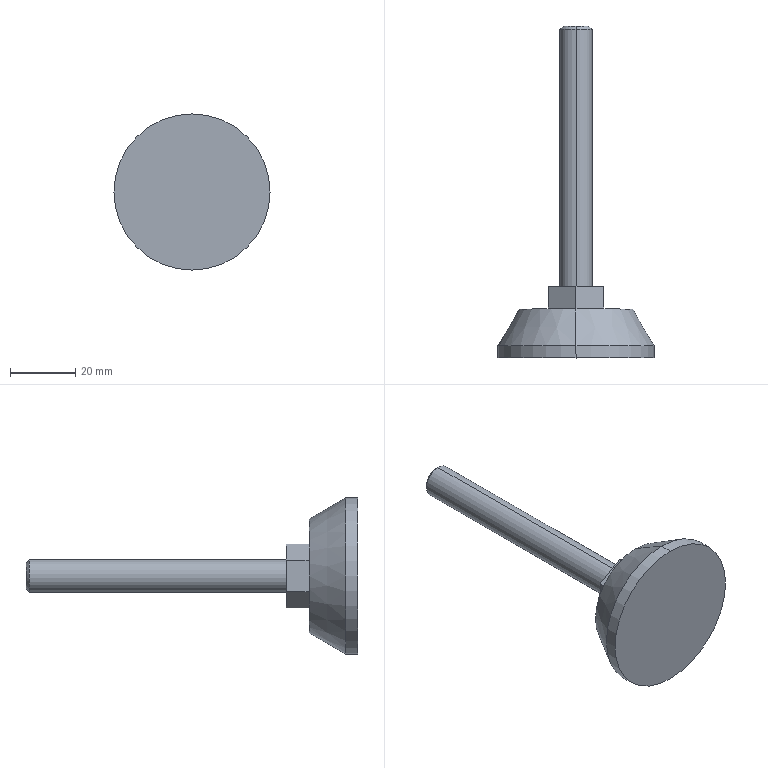Part | STEP file | AJC-D48-M10-L80 | 1 solid | 18 faces | box 48 x 102 x 48 mm | volume 30151 mm3 | plane 10 | cylinder 4 | cone 4 | commonest cylinder face diameters 10 x2 48 x2
STEP:
#1=CARTESIAN_POINT('',(0.,3.75,-24.));
#2=VERTEX_POINT('',#1);
#3=CARTESIAN_POINT('',(0.,3.75,24.));
#4=VERTEX_POINT('',#3);
#5=CARTESIAN_POINT('',(0.,3.75,0.));
#6=DIRECTION('',(0.,-1.,0.));
#7=DIRECTION('',(0.,0.,-1.));
#8=AXIS2_PLACEMENT_3D('',#5,#6,#7);
#9=CIRCLE('',#8,24.);
#10=EDGE_CURVE('',#2,#4,#9,.T.);
#11=ORIENTED_EDGE('',*,*,#10,.T.);
#12=CARTESIAN_POINT('',(0.,0.,24.));
#13=VERTEX_POINT('',#12);
#14=CARTESIAN_POINT('',(0.,107.1,24.));
#15=DIRECTION('',(0.,-1.,0.));
#16=VECTOR('',#15,1000.);
#17=LINE('',#14,#16);
#18=EDGE_CURVE('',#4,#13,#17,.T.);
#19=ORIENTED_EDGE('',*,*,#18,.T.);
#20=CARTESIAN_POINT('',(0.,0.,-24.));
#21=VERTEX_POINT('',#20);
#22=CARTESIAN_POINT('',(0.,0.,0.));
#23=DIRECTION('',(0.,-1.,0.));
#24=DIRECTION('',(0.,0.,-1.));
#25=AXIS2_PLACEMENT_3D('',#22,#23,#24);
#26=CIRCLE('',#25,24.);
#27=EDGE_CURVE('',#21,#13,#26,.T.);
#28=ORIENTED_EDGE('',*,*,#27,.F.);
#29=CARTESIAN_POINT('',(0.,107.1,-24.));
#30=DIRECTION('',(0.,-1.,0.));
#31=VECTOR('',#30,1000.);
#32=LINE('',#29,#31);
#33=EDGE_CURVE('',#2,#21,#32,.T.);
#34=ORIENTED_EDGE('',*,*,#33,.F.);
#35=EDGE_LOOP('',(#11,#19,#28,#34));
#36=FACE_OUTER_BOUND('',#35,.T.);
#37=CARTESIAN_POINT('',(0.,107.1,0.));
#38=DIRECTION('',(0.,-1.,0.));
#39=DIRECTION('',(0.,0.,-1.));
#40=AXIS2_PLACEMENT_3D('',#37,#38,#39);
#41=CYLINDRICAL_SURFACE('',#40,24.);
#42=ADVANCED_FACE('',(#36),#41,.T.);
#43=CARTESIAN_POINT('',(0.,15.,-17.505));
#44=VERTEX_POINT('',#43);
#45=CARTESIAN_POINT('',(0.,15.,17.505));
#46=VERTEX_POINT('',#45);
#47=CARTESIAN_POINT('',(0.,15.,0.));
#48=DIRECTION('',(0.,-1.,0.));
#49=DIRECTION('',(0.,0.,-1.));
#50=AXIS2_PLACEMENT_3D('',#47,#48,#49);
#51=CIRCLE('',#50,17.505);
#52=EDGE_CURVE('',#44,#46,#51,.T.);
#53=ORIENTED_EDGE('',*,*,#52,.T.);
#54=CARTESIAN_POINT('',(0.,3.75,24.));
#55=DIRECTION('',(0.,-0.866,0.5));
#56=VECTOR('',#55,1000.);
#57=LINE('',#54,#56);
#58=EDGE_CURVE('',#46,#4,#57,.T.);
#59=ORIENTED_EDGE('',*,*,#58,.T.);
#60=ORIENTED_EDGE('',*,*,#10,.F.);
#61=CARTESIAN_POINT('',(0.,3.75,-24.));
#62=DIRECTION('',(0.,-0.866,-0.5));
#63=VECTOR('',#62,1000.);
#64=LINE('',#61,#63);
#65=EDGE_CURVE('',#44,#2,#64,.T.);
#66=ORIENTED_EDGE('',*,*,#65,.F.);
#67=EDGE_LOOP('',(#53,#59,#60,#66));
#68=FACE_OUTER_BOUND('',#67,.T.);
#69=CARTESIAN_POINT('',(0.,3.75,0.));
#70=DIRECTION('',(0.,-1.,0.));
#71=DIRECTION('',(0.,0.,-1.));
#72=AXIS2_PLACEMENT_3D('',#69,#70,#71);
#73=CONICAL_SURFACE('',#72,24.,0.5236);
#74=ADVANCED_FACE('',(#68),#73,.T.);
#75=CARTESIAN_POINT('',(0.,101.,-5.));
#76=VERTEX_POINT('',#75);
#77=CARTESIAN_POINT('',(0.,101.,5.));
#78=VERTEX_POINT('',#77);
#79=CARTESIAN_POINT('',(0.,101.,0.));
#80=DIRECTION('',(0.,-1.,0.));
#81=DIRECTION('',(0.,0.,-1.));
#82=AXIS2_PLACEMENT_3D('',#79,#80,#81);
#83=CIRCLE('',#82,5.);
#84=EDGE_CURVE('',#76,#78,#83,.T.);
#85=ORIENTED_EDGE('',*,*,#84,.T.);
#86=CARTESIAN_POINT('',(0.,22.,5.));
#87=VERTEX_POINT('',#86);
#88=CARTESIAN_POINT('',(0.,107.1,5.));
#89=DIRECTION('',(0.,-1.,0.));
#90=VECTOR('',#89,1000.);
#91=LINE('',#88,#90);
#92=EDGE_CURVE('',#78,#87,#91,.T.);
#93=ORIENTED_EDGE('',*,*,#92,.T.);
#94=CARTESIAN_POINT('',(0.,22.,-5.));
#95=VERTEX_POINT('',#94);
#96=CARTESIAN_POINT('',(0.,22.,0.));
#97=DIRECTION('',(0.,1.,0.));
#98=DIRECTION('',(0.,0.,-1.));
#99=AXIS2_PLACEMENT_3D('',#96,#97,#98);
#100=CIRCLE('',#99,5.);
#101=EDGE_CURVE('',#87,#95,#100,.T.);
#102=ORIENTED_EDGE('',*,*,#101,.T.);
#103=CARTESIAN_POINT('',(0.,107.1,-5.));
#104=DIRECTION('',(0.,-1.,0.));
#105=VECTOR('',#104,1000.);
#106=LINE('',#103,#105);
#107=EDGE_CURVE('',#76,#95,#106,.T.);
#108=ORIENTED_EDGE('',*,*,#107,.F.);
#109=EDGE_LOOP('',(#85,#93,#102,#108));
#110=FACE_OUTER_BOUND('',#109,.T.);
#111=CARTESIAN_POINT('',(0.,107.1,0.));
#112=DIRECTION('',(0.,-1.,0.));
#113=DIRECTION('',(0.,0.,-1.));
#114=AXIS2_PLACEMENT_3D('',#111,#112,#113);
#115=CYLINDRICAL_SURFACE('',#114,5.);
#116=ADVANCED_FACE('',(#110),#115,.T.);
#117=CARTESIAN_POINT('',(0.,102.,-4.));
#118=VERTEX_POINT('',#117);
#119=CARTESIAN_POINT('',(0.,102.,4.));
#120=VERTEX_POINT('',#119);
#121=CARTESIAN_POINT('',(0.,102.,0.));
#122=DIRECTION('',(0.,-1.,0.));
#123=DIRECTION('',(0.,0.,-1.));
#124=AXIS2_PLACEMENT_3D('',#121,#122,#123);
#125=CIRCLE('',#124,4.);
#126=EDGE_CURVE('',#118,#120,#125,.T.);
#127=ORIENTED_EDGE('',*,*,#126,.T.);
#128=CARTESIAN_POINT('',(0.,101.,5.));
#129=DIRECTION('',(0.,-0.7071,0.7071));
#130=VECTOR('',#129,1000.);
#131=LINE('',#128,#130);
#132=EDGE_CURVE('',#120,#78,#131,.T.);
#133=ORIENTED_EDGE('',*,*,#132,.T.);
#134=ORIENTED_EDGE('',*,*,#84,.F.);
#135=CARTESIAN_POINT('',(0.,101.,-5.));
#136=DIRECTION('',(0.,-0.7071,-0.7071));
#137=VECTOR('',#136,1000.);
#138=LINE('',#135,#137);
#139=EDGE_CURVE('',#118,#76,#138,.T.);
#140=ORIENTED_EDGE('',*,*,#139,.F.);
#141=EDGE_LOOP('',(#127,#133,#134,#140));
#142=FACE_OUTER_BOUND('',#141,.T.);
#143=CARTESIAN_POINT('',(0.,101.,0.));
#144=DIRECTION('',(0.,-1.,0.));
#145=DIRECTION('',(0.,0.,-1.));
#146=AXIS2_PLACEMENT_3D('',#143,#144,#145);
#147=CONICAL_SURFACE('',#146,5.,0.7854);
#148=ADVANCED_FACE('',(#142),#147,.T.);
#149=ORIENTED_EDGE('',*,*,#27,.T.);
#150=CARTESIAN_POINT('',(0.,0.,0.));
#151=DIRECTION('',(0.,-1.,0.));
#152=DIRECTION('',(0.,0.,-1.));
#153=AXIS2_PLACEMENT_3D('',#150,#151,#152);
#154=CIRCLE('',#153,24.);
#155=EDGE_CURVE('',#13,#21,#154,.T.);
#156=ORIENTED_EDGE('',*,*,#155,.T.);
#157=EDGE_LOOP('',(#149,#156));
#158=FACE_OUTER_BOUND('',#157,.T.);
#159=CARTESIAN_POINT('',(0.,0.,0.));
#160=DIRECTION('',(0.,-1.,0.));
#161=DIRECTION('',(0.,0.,-1.));
#162=AXIS2_PLACEMENT_3D('',#159,#160,#161);
#163=PLANE('',#162);
#164=ADVANCED_FACE('',(#158),#163,.T.);
#165=ORIENTED_EDGE('',*,*,#18,.F.);
#166=CARTESIAN_POINT('',(0.,3.75,0.));
#167=DIRECTION('',(0.,-1.,0.));
#168=DIRECTION('',(0.,0.,-1.));
#169=AXIS2_PLACEMENT_3D('',#166,#167,#168);
#170=CIRCLE('',#169,24.);
#171=EDGE_CURVE('',#4,#2,#170,.T.);
#172=ORIENTED_EDGE('',*,*,#171,.T.);
#173=ORIENTED_EDGE('',*,*,#33,.T.);
#174=ORIENTED_EDGE('',*,*,#155,.F.);
#175=EDGE_LOOP('',(#165,#172,#173,#174));
#176=FACE_OUTER_BOUND('',#175,.T.);
#177=CARTESIAN_POINT('',(0.,107.1,0.));
#178=DIRECTION('',(0.,-1.,0.));
#179=DIRECTION('',(0.,0.,-1.));
#180=AXIS2_PLACEMENT_3D('',#177,#178,#179);
#181=CYLINDRICAL_SURFACE('',#180,24.);
#182=ADVANCED_FACE('',(#176),#181,.T.);
#183=ORIENTED_EDGE('',*,*,#58,.F.);
#184=CARTESIAN_POINT('',(0.,15.,0.));
#185=DIRECTION('',(0.,-1.,0.));
#186=DIRECTION('',(0.,0.,-1.));
#187=AXIS2_PLACEMENT_3D('',#184,#185,#186);
#188=CIRCLE('',#187,17.505);
#189=EDGE_CURVE('',#46,#44,#188,.T.);
#190=ORIENTED_EDGE('',*,*,#189,.T.);
#191=ORIENTED_EDGE('',*,*,#65,.T.);
#192=ORIENTED_EDGE('',*,*,#171,.F.);
#193=EDGE_LOOP('',(#183,#190,#191,#192));
#194=FACE_OUTER_BOUND('',#193,.T.);
#195=CARTESIAN_POINT('',(0.,3.75,0.));
#196=DIRECTION('',(0.,-1.,0.));
#197=DIRECTION('',(0.,0.,-1.));
#198=AXIS2_PLACEMENT_3D('',#195,#196,#197);
#199=CONICAL_SURFACE('',#198,24.,0.5236);
#200=ADVANCED_FACE('',(#194),#199,.T.);
#201=CARTESIAN_POINT('',(8.5,15.,4.907));
#202=VERTEX_POINT('',#201);
#203=CARTESIAN_POINT('',(8.5,15.,-4.907));
#204=VERTEX_POINT('',#203);
#205=CARTESIAN_POINT('',(8.5,15.,0.));
#206=DIRECTION('',(0.,0.,-1.));
#207=VECTOR('',#206,1000.);
#208=LINE('',#205,#207);
#209=EDGE_CURVE('',#202,#204,#208,.T.);
#210=ORIENTED_EDGE('',*,*,#209,.F.);
#211=CARTESIAN_POINT('',(0.,15.,9.815));
#212=VERTEX_POINT('',#211);
#213=CARTESIAN_POINT('',(0.,15.,9.815));
#214=DIRECTION('',(0.866,0.,-0.5));
#215=VECTOR('',#214,1000.);
#216=LINE('',#213,#215);
#217=EDGE_CURVE('',#212,#202,#216,.T.);
#218=ORIENTED_EDGE('',*,*,#217,.F.);
#219=CARTESIAN_POINT('',(-8.5,15.,4.907));
#220=VERTEX_POINT('',#219);
#221=CARTESIAN_POINT('',(-8.5,15.,4.907));
#222=DIRECTION('',(0.866,0.,0.5));
#223=VECTOR('',#222,1000.);
#224=LINE('',#221,#223);
#225=EDGE_CURVE('',#220,#212,#224,.T.);
#226=ORIENTED_EDGE('',*,*,#225,.F.);
#227=CARTESIAN_POINT('',(-8.5,15.,-4.907));
#228=VERTEX_POINT('',#227);
#229=CARTESIAN_POINT('',(-8.5,15.,0.));
#230=DIRECTION('',(0.,0.,1.));
#231=VECTOR('',#230,1000.);
#232=LINE('',#229,#231);
#233=EDGE_CURVE('',#228,#220,#232,.T.);
#234=ORIENTED_EDGE('',*,*,#233,.F.);
#235=CARTESIAN_POINT('',(0.,15.,-9.815));
#236=VERTEX_POINT('',#235);
#237=CARTESIAN_POINT('',(0.,15.,-9.815));
#238=DIRECTION('',(-0.866,0.,0.5));
#239=VECTOR('',#238,1000.);
#240=LINE('',#237,#239);
#241=EDGE_CURVE('',#236,#228,#240,.T.);
#242=ORIENTED_EDGE('',*,*,#241,.F.);
#243=CARTESIAN_POINT('',(8.5,15.,-4.907));
#244=DIRECTION('',(-0.866,0.,-0.5));
#245=VECTOR('',#244,1000.);
#246=LINE('',#243,#245);
#247=EDGE_CURVE('',#204,#236,#246,.T.);
#248=ORIENTED_EDGE('',*,*,#247,.F.);
#249=EDGE_LOOP('',(#210,#218,#226,#234,#242,#248));
#250=FACE_BOUND('',#249,.T.);
#251=ORIENTED_EDGE('',*,*,#52,.F.);
#252=ORIENTED_EDGE('',*,*,#189,.F.);
#253=EDGE_LOOP('',(#251,#252));
#254=FACE_OUTER_BOUND('',#253,.T.);
#255=CARTESIAN_POINT('',(0.,15.,0.));
#256=DIRECTION('',(0.,-1.,0.));
#257=DIRECTION('',(0.,0.,-1.));
#258=AXIS2_PLACEMENT_3D('',#255,#256,#257);
#259=PLANE('',#258);
#260=ADVANCED_FACE('',(#250,#254),#259,.F.);
#261=CARTESIAN_POINT('',(8.5,22.,-4.907));
#262=VERTEX_POINT('',#261);
#263=CARTESIAN_POINT('',(8.5,22.,-4.907));
#264=DIRECTION('',(0.,-1.,0.));
#265=VECTOR('',#264,1000.);
#266=LINE('',#263,#265);
#267=EDGE_CURVE('',#262,#204,#266,.T.);
#268=ORIENTED_EDGE('',*,*,#267,.T.);
#269=ORIENTED_EDGE('',*,*,#247,.T.);
#270=CARTESIAN_POINT('',(0.,22.,-9.815));
#271=VERTEX_POINT('',#270);
#272=CARTESIAN_POINT('',(0.,22.,-9.815));
#273=DIRECTION('',(0.,1.,0.));
#274=VECTOR('',#273,1000.);
#275=LINE('',#272,#274);
#276=EDGE_CURVE('',#236,#271,#275,.T.);
#277=ORIENTED_EDGE('',*,*,#276,.T.);
#278=CARTESIAN_POINT('',(8.5,22.,-4.907));
#279=DIRECTION('',(0.866,0.,0.5));
#280=VECTOR('',#279,1000.);
#281=LINE('',#278,#280);
#282=EDGE_CURVE('',#271,#262,#281,.T.);
#283=ORIENTED_EDGE('',*,*,#282,.T.);
#284=EDGE_LOOP('',(#268,#269,#277,#283));
#285=FACE_OUTER_BOUND('',#284,.T.);
#286=CARTESIAN_POINT('',(8.5,22.,-4.907));
#287=DIRECTION('',(0.5,0.,-0.866));
#288=DIRECTION('',(-0.866,0.,-0.5));
#289=AXIS2_PLACEMENT_3D('',#286,#287,#288);
#290=PLANE('',#289);
#291=ADVANCED_FACE('',(#285),#290,.T.);
#292=CARTESIAN_POINT('',(8.5,22.,4.907));
#293=VERTEX_POINT('',#292);
#294=CARTESIAN_POINT('',(8.5,22.,4.907));
#295=DIRECTION('',(0.,-1.,0.));
#296=VECTOR('',#295,1000.);
#297=LINE('',#294,#296);
#298=EDGE_CURVE('',#293,#202,#297,.T.);
#299=ORIENTED_EDGE('',*,*,#298,.T.);
#300=ORIENTED_EDGE('',*,*,#209,.T.);
#301=ORIENTED_EDGE('',*,*,#267,.F.);
#302=CARTESIAN_POINT('',(8.5,22.,4.907));
#303=DIRECTION('',(0.,0.,1.));
#304=VECTOR('',#303,1000.);
#305=LINE('',#302,#304);
#306=EDGE_CURVE('',#262,#293,#305,.T.);
#307=ORIENTED_EDGE('',*,*,#306,.T.);
#308=EDGE_LOOP('',(#299,#300,#301,#307));
#309=FACE_OUTER_BOUND('',#308,.T.);
#310=CARTESIAN_POINT('',(8.5,22.,4.907));
#311=DIRECTION('',(1.,0.,0.));
#312=DIRECTION('',(0.,0.,-1.));
#313=AXIS2_PLACEMENT_3D('',#310,#311,#312);
#314=PLANE('',#313);
#315=ADVANCED_FACE('',(#309),#314,.T.);
#316=CARTESIAN_POINT('',(0.,22.,9.815));
#317=VERTEX_POINT('',#316);
#318=CARTESIAN_POINT('',(0.,22.,9.815));
#319=DIRECTION('',(0.,-1.,0.));
#320=VECTOR('',#319,1000.);
#321=LINE('',#318,#320);
#322=EDGE_CURVE('',#317,#212,#321,.T.);
#323=ORIENTED_EDGE('',*,*,#322,.T.);
#324=ORIENTED_EDGE('',*,*,#217,.T.);
#325=ORIENTED_EDGE('',*,*,#298,.F.);
#326=CARTESIAN_POINT('',(0.,22.,9.815));
#327=DIRECTION('',(-0.866,0.,0.5));
#328=VECTOR('',#327,1000.);
#329=LINE('',#326,#328);
#330=EDGE_CURVE('',#293,#317,#329,.T.);
#331=ORIENTED_EDGE('',*,*,#330,.T.);
#332=EDGE_LOOP('',(#323,#324,#325,#331));
#333=FACE_OUTER_BOUND('',#332,.T.);
#334=CARTESIAN_POINT('',(0.,22.,9.815));
#335=DIRECTION('',(0.5,0.,0.866));
#336=DIRECTION('',(0.866,0.,-0.5));
#337=AXIS2_PLACEMENT_3D('',#334,#335,#336);
#338=PLANE('',#337);
#339=ADVANCED_FACE('',(#333),#338,.T.);
#340=CARTESIAN_POINT('',(-8.5,22.,4.907));
#341=VERTEX_POINT('',#340);
#342=CARTESIAN_POINT('',(-8.5,22.,4.907));
#343=DIRECTION('',(0.,-1.,0.));
#344=VECTOR('',#343,1000.);
#345=LINE('',#342,#344);
#346=EDGE_CURVE('',#341,#220,#345,.T.);
#347=ORIENTED_EDGE('',*,*,#346,.T.);
#348=ORIENTED_EDGE('',*,*,#225,.T.);
#349=ORIENTED_EDGE('',*,*,#322,.F.);
#350=CARTESIAN_POINT('',(-8.5,22.,4.907));
#351=DIRECTION('',(-0.866,0.,-0.5));
#352=VECTOR('',#351,1000.);
#353=LINE('',#350,#352);
#354=EDGE_CURVE('',#317,#341,#353,.T.);
#355=ORIENTED_EDGE('',*,*,#354,.T.);
#356=EDGE_LOOP('',(#347,#348,#349,#355));
#357=FACE_OUTER_BOUND('',#356,.T.);
#358=CARTESIAN_POINT('',(-8.5,22.,4.907));
#359=DIRECTION('',(-0.5,0.,0.866));
#360=DIRECTION('',(0.866,0.,0.5));
#361=AXIS2_PLACEMENT_3D('',#358,#359,#360);
#362=PLANE('',#361);
#363=ADVANCED_FACE('',(#357),#362,.T.);
#364=CARTESIAN_POINT('',(-8.5,22.,-4.907));
#365=VERTEX_POINT('',#364);
#366=CARTESIAN_POINT('',(-8.5,22.,-4.907));
#367=DIRECTION('',(0.,-1.,0.));
#368=VECTOR('',#367,1000.);
#369=LINE('',#366,#368);
#370=EDGE_CURVE('',#365,#228,#369,.T.);
#371=ORIENTED_EDGE('',*,*,#370,.T.);
#372=ORIENTED_EDGE('',*,*,#233,.T.);
#373=ORIENTED_EDGE('',*,*,#346,.F.);
#374=CARTESIAN_POINT('',(-8.5,22.,-4.907));
#375=DIRECTION('',(0.,0.,-1.));
#376=VECTOR('',#375,1000.);
#377=LINE('',#374,#376);
#378=EDGE_CURVE('',#341,#365,#377,.T.);
#379=ORIENTED_EDGE('',*,*,#378,.T.);
#380=EDGE_LOOP('',(#371,#372,#373,#379));
#381=FACE_OUTER_BOUND('',#380,.T.);
#382=CARTESIAN_POINT('',(-8.5,22.,-4.907));
#383=DIRECTION('',(-1.,0.,0.));
#384=DIRECTION('',(0.,0.,1.));
#385=AXIS2_PLACEMENT_3D('',#382,#383,#384);
#386=PLANE('',#385);
#387=ADVANCED_FACE('',(#381),#386,.T.);
#388=ORIENTED_EDGE('',*,*,#276,.F.);
#389=ORIENTED_EDGE('',*,*,#241,.T.);
#390=ORIENTED_EDGE('',*,*,#370,.F.);
#391=CARTESIAN_POINT('',(0.,22.,-9.815));
#392=DIRECTION('',(0.866,0.,-0.5));
#393=VECTOR('',#392,1000.);
#394=LINE('',#391,#393);
#395=EDGE_CURVE('',#365,#271,#394,.T.);
#396=ORIENTED_EDGE('',*,*,#395,.T.);
#397=EDGE_LOOP('',(#388,#389,#390,#396));
#398=FACE_OUTER_BOUND('',#397,.T.);
#399=CARTESIAN_POINT('',(0.,22.,-9.815));
#400=DIRECTION('',(-0.5,0.,-0.866));
#401=DIRECTION('',(-0.866,0.,0.5));
#402=AXIS2_PLACEMENT_3D('',#399,#400,#401);
#403=PLANE('',#402);
#404=ADVANCED_FACE('',(#398),#403,.T.);
#405=CARTESIAN_POINT('',(0.,22.,0.));
#406=DIRECTION('',(0.,1.,0.));
#407=DIRECTION('',(0.,0.,-1.));
#408=AXIS2_PLACEMENT_3D('',#405,#406,#407);
#409=CIRCLE('',#408,5.);
#410=EDGE_CURVE('',#95,#87,#409,.T.);
#411=ORIENTED_EDGE('',*,*,#410,.F.);
#412=ORIENTED_EDGE('',*,*,#101,.F.);
#413=EDGE_LOOP('',(#411,#412));
#414=FACE_BOUND('',#413,.T.);
#415=ORIENTED_EDGE('',*,*,#306,.F.);
#416=ORIENTED_EDGE('',*,*,#282,.F.);
#417=ORIENTED_EDGE('',*,*,#395,.F.);
#418=ORIENTED_EDGE('',*,*,#378,.F.);
#419=ORIENTED_EDGE('',*,*,#354,.F.);
#420=ORIENTED_EDGE('',*,*,#330,.F.);
#421=EDGE_LOOP('',(#415,#416,#417,#418,#419,#420));
#422=FACE_OUTER_BOUND('',#421,.T.);
#423=CARTESIAN_POINT('',(0.,22.,0.));
#424=DIRECTION('',(0.,-1.,0.));
#425=DIRECTION('',(0.,0.,-1.));
#426=AXIS2_PLACEMENT_3D('',#423,#424,#425);
#427=PLANE('',#426);
#428=ADVANCED_FACE('',(#414,#422),#427,.F.);
#429=ORIENTED_EDGE('',*,*,#92,.F.);
#430=CARTESIAN_POINT('',(0.,101.,0.));
#431=DIRECTION('',(0.,-1.,0.));
#432=DIRECTION('',(0.,0.,-1.));
#433=AXIS2_PLACEMENT_3D('',#430,#431,#432);
#434=CIRCLE('',#433,5.);
#435=EDGE_CURVE('',#78,#76,#434,.T.);
#436=ORIENTED_EDGE('',*,*,#435,.T.);
#437=ORIENTED_EDGE('',*,*,#107,.T.);
#438=ORIENTED_EDGE('',*,*,#410,.T.);
#439=EDGE_LOOP('',(#429,#436,#437,#438));
#440=FACE_OUTER_BOUND('',#439,.T.);
#441=CARTESIAN_POINT('',(0.,107.1,0.));
#442=DIRECTION('',(0.,-1.,0.));
#443=DIRECTION('',(0.,0.,-1.));
#444=AXIS2_PLACEMENT_3D('',#441,#442,#443);
#445=CYLINDRICAL_SURFACE('',#444,5.);
#446=ADVANCED_FACE('',(#440),#445,.T.);
#447=ORIENTED_EDGE('',*,*,#132,.F.);
#448=CARTESIAN_POINT('',(0.,102.,0.));
#449=DIRECTION('',(0.,-1.,0.));
#450=DIRECTION('',(0.,0.,-1.));
#451=AXIS2_PLACEMENT_3D('',#448,#449,#450);
#452=CIRCLE('',#451,4.);
#453=EDGE_CURVE('',#120,#118,#452,.T.);
#454=ORIENTED_EDGE('',*,*,#453,.T.);
#455=ORIENTED_EDGE('',*,*,#139,.T.);
#456=ORIENTED_EDGE('',*,*,#435,.F.);
#457=EDGE_LOOP('',(#447,#454,#455,#456));
#458=FACE_OUTER_BOUND('',#457,.T.);
#459=CARTESIAN_POINT('',(0.,101.,0.));
#460=DIRECTION('',(0.,-1.,0.));
#461=DIRECTION('',(0.,0.,-1.));
#462=AXIS2_PLACEMENT_3D('',#459,#460,#461);
#463=CONICAL_SURFACE('',#462,5.,0.7854);
#464=ADVANCED_FACE('',(#458),#463,.T.);
#465=ORIENTED_EDGE('',*,*,#126,.F.);
#466=ORIENTED_EDGE('',*,*,#453,.F.);
#467=EDGE_LOOP('',(#465,#466));
#468=FACE_OUTER_BOUND('',#467,.T.);
#469=CARTESIAN_POINT('',(0.,102.,0.));
#470=DIRECTION('',(0.,-1.,0.));
#471=DIRECTION('',(0.,0.,-1.));
#472=AXIS2_PLACEMENT_3D('',#469,#470,#471);
#473=PLANE('',#472);
#474=ADVANCED_FACE('',(#468),#473,.F.);
#475=CLOSED_SHELL('',(#42,#74,#116,#148,#164,#182,#200,#260,#291,#315,#339,#363,#387,#404,#428,#446,#464,#474));
#476=MANIFOLD_SOLID_BREP('',#475);
#477=CARTESIAN_POINT('',(0.,0.,0.));
#478=DIRECTION('',(0.,0.,1.));
#479=DIRECTION('',(1.,0.,0.));
#480=AXIS2_PLACEMENT_3D('',#477,#478,#479);
#481=(LENGTH_UNIT()NAMED_UNIT(*)SI_UNIT(.MILLI.,.METRE.));
#482=UNCERTAINTY_MEASURE_WITH_UNIT(LENGTH_MEASURE(0.00001),#481,'','');
#483=(NAMED_UNIT(*)PLANE_ANGLE_UNIT()SI_UNIT($,.RADIAN.));
#484=(NAMED_UNIT(*)SI_UNIT($,.STERADIAN.)SOLID_ANGLE_UNIT());
#485=(GEOMETRIC_REPRESENTATION_CONTEXT(3)GLOBAL_UNCERTAINTY_ASSIGNED_CONTEXT((#482))GLOBAL_UNIT_ASSIGNED_CONTEXT((#481,#483,#484))REPRESENTATION_CONTEXT('',''));
#486=ADVANCED_BREP_SHAPE_REPRESENTATION('',(#476,#480),#485);